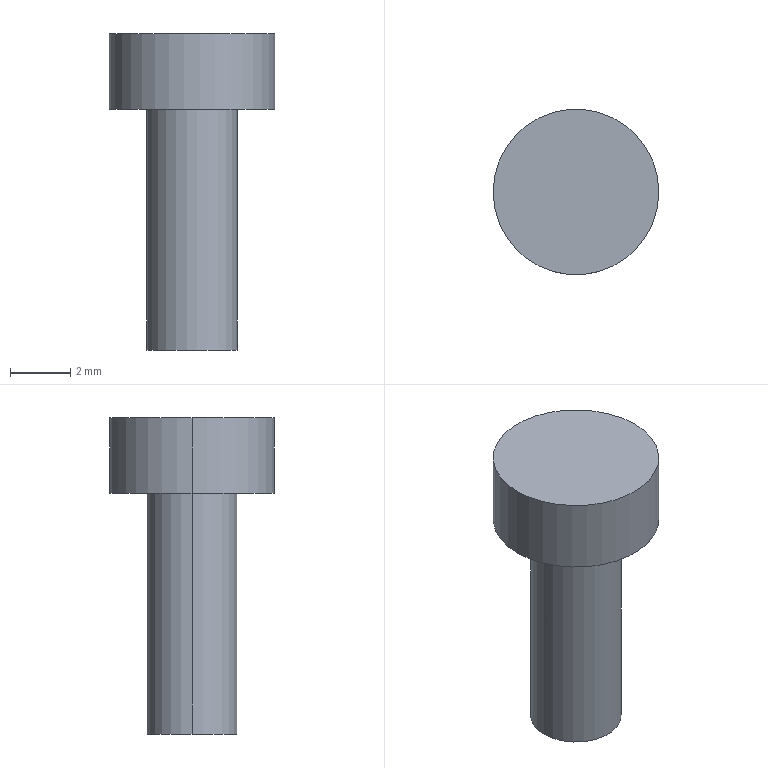Part | SolidWorks | features Extrusion 1, ICE 1 | 1 solid | 7 faces | box 5.5 x 5.5 x 10.5 mm | volume 115.944 mm3 | cylinder 4 | plane 3 | commonest cylinder face diameters 3 x2 5.5 x2
STEP:
#1=CARTESIAN_POINT('',(2.75,0.,2.5));
#2=VERTEX_POINT('',#1);
#3=CARTESIAN_POINT('',(-2.75,0.,2.5));
#4=VERTEX_POINT('',#3);
#5=CARTESIAN_POINT('',(0.,0.,2.5));
#6=DIRECTION('',(0.,0.,1.));
#7=DIRECTION('',(1.,0.,0.));
#8=AXIS2_PLACEMENT_3D('',#5,#6,#7);
#9=CIRCLE('',#8,2.75);
#10=EDGE_CURVE('',#2,#4,#9,.T.);
#11=ORIENTED_EDGE('',*,*,#10,.F.);
#12=CARTESIAN_POINT('',(2.75,0.,0.));
#13=VERTEX_POINT('',#12);
#14=CARTESIAN_POINT('',(2.75,0.,2.5));
#15=DIRECTION('',(0.,0.,-1.));
#16=VECTOR('',#15,1000.);
#17=LINE('',#14,#16);
#18=EDGE_CURVE('',#2,#13,#17,.T.);
#19=ORIENTED_EDGE('',*,*,#18,.T.);
#20=CARTESIAN_POINT('',(-2.75,0.,0.));
#21=VERTEX_POINT('',#20);
#22=CARTESIAN_POINT('',(0.,0.,0.));
#23=DIRECTION('',(0.,0.,1.));
#24=DIRECTION('',(1.,0.,0.));
#25=AXIS2_PLACEMENT_3D('',#22,#23,#24);
#26=CIRCLE('',#25,2.75);
#27=EDGE_CURVE('',#13,#21,#26,.T.);
#28=ORIENTED_EDGE('',*,*,#27,.T.);
#29=CARTESIAN_POINT('',(-2.75,0.,2.5));
#30=DIRECTION('',(0.,0.,-1.));
#31=VECTOR('',#30,1000.);
#32=LINE('',#29,#31);
#33=EDGE_CURVE('',#4,#21,#32,.T.);
#34=ORIENTED_EDGE('',*,*,#33,.F.);
#35=EDGE_LOOP('',(#11,#19,#28,#34));
#36=FACE_OUTER_BOUND('',#35,.T.);
#37=CARTESIAN_POINT('',(0.,0.,2.5));
#38=DIRECTION('',(0.,0.,-1.));
#39=DIRECTION('',(-1.,0.,0.));
#40=AXIS2_PLACEMENT_3D('',#37,#38,#39);
#41=CYLINDRICAL_SURFACE('',#40,2.75);
#42=ADVANCED_FACE('',(#36),#41,.T.);
#43=CARTESIAN_POINT('',(1.5,0.,-8.));
#44=VERTEX_POINT('',#43);
#45=CARTESIAN_POINT('',(-1.5,0.,-8.));
#46=VERTEX_POINT('',#45);
#47=CARTESIAN_POINT('',(0.,0.,-8.));
#48=DIRECTION('',(0.,0.,1.));
#49=DIRECTION('',(1.,0.,0.));
#50=AXIS2_PLACEMENT_3D('',#47,#48,#49);
#51=CIRCLE('',#50,1.5);
#52=EDGE_CURVE('',#44,#46,#51,.T.);
#53=ORIENTED_EDGE('',*,*,#52,.T.);
#54=CARTESIAN_POINT('',(-1.5,0.,0.));
#55=VERTEX_POINT('',#54);
#56=CARTESIAN_POINT('',(-1.5,0.,-8.));
#57=DIRECTION('',(0.,0.,1.));
#58=VECTOR('',#57,1000.);
#59=LINE('',#56,#58);
#60=EDGE_CURVE('',#46,#55,#59,.T.);
#61=ORIENTED_EDGE('',*,*,#60,.T.);
#62=CARTESIAN_POINT('',(1.5,0.,0.));
#63=VERTEX_POINT('',#62);
#64=CARTESIAN_POINT('',(0.,0.,0.));
#65=DIRECTION('',(0.,0.,1.));
#66=DIRECTION('',(1.,0.,0.));
#67=AXIS2_PLACEMENT_3D('',#64,#65,#66);
#68=CIRCLE('',#67,1.5);
#69=EDGE_CURVE('',#63,#55,#68,.T.);
#70=ORIENTED_EDGE('',*,*,#69,.F.);
#71=CARTESIAN_POINT('',(1.5,0.,-8.));
#72=DIRECTION('',(0.,0.,1.));
#73=VECTOR('',#72,1000.);
#74=LINE('',#71,#73);
#75=EDGE_CURVE('',#44,#63,#74,.T.);
#76=ORIENTED_EDGE('',*,*,#75,.F.);
#77=EDGE_LOOP('',(#53,#61,#70,#76));
#78=FACE_OUTER_BOUND('',#77,.T.);
#79=CARTESIAN_POINT('',(0.,0.,-8.));
#80=DIRECTION('',(0.,0.,1.));
#81=DIRECTION('',(1.,0.,0.));
#82=AXIS2_PLACEMENT_3D('',#79,#80,#81);
#83=CYLINDRICAL_SURFACE('',#82,1.5);
#84=ADVANCED_FACE('',(#78),#83,.T.);
#85=ORIENTED_EDGE('',*,*,#60,.F.);
#86=CARTESIAN_POINT('',(0.,0.,-8.));
#87=DIRECTION('',(0.,0.,1.));
#88=DIRECTION('',(1.,0.,0.));
#89=AXIS2_PLACEMENT_3D('',#86,#87,#88);
#90=CIRCLE('',#89,1.5);
#91=EDGE_CURVE('',#46,#44,#90,.T.);
#92=ORIENTED_EDGE('',*,*,#91,.T.);
#93=ORIENTED_EDGE('',*,*,#75,.T.);
#94=CARTESIAN_POINT('',(0.,0.,0.));
#95=DIRECTION('',(0.,0.,1.));
#96=DIRECTION('',(1.,0.,0.));
#97=AXIS2_PLACEMENT_3D('',#94,#95,#96);
#98=CIRCLE('',#97,1.5);
#99=EDGE_CURVE('',#55,#63,#98,.T.);
#100=ORIENTED_EDGE('',*,*,#99,.F.);
#101=EDGE_LOOP('',(#85,#92,#93,#100));
#102=FACE_OUTER_BOUND('',#101,.T.);
#103=CARTESIAN_POINT('',(0.,0.,-8.));
#104=DIRECTION('',(0.,0.,1.));
#105=DIRECTION('',(1.,0.,0.));
#106=AXIS2_PLACEMENT_3D('',#103,#104,#105);
#107=CYLINDRICAL_SURFACE('',#106,1.5);
#108=ADVANCED_FACE('',(#102),#107,.T.);
#109=ORIENTED_EDGE('',*,*,#52,.F.);
#110=ORIENTED_EDGE('',*,*,#91,.F.);
#111=EDGE_LOOP('',(#109,#110));
#112=FACE_OUTER_BOUND('',#111,.T.);
#113=CARTESIAN_POINT('',(0.,0.,-8.));
#114=DIRECTION('',(0.,0.,1.));
#115=DIRECTION('',(1.,0.,0.));
#116=AXIS2_PLACEMENT_3D('',#113,#114,#115);
#117=PLANE('',#116);
#118=ADVANCED_FACE('',(#112),#117,.F.);
#119=ORIENTED_EDGE('',*,*,#18,.F.);
#120=CARTESIAN_POINT('',(0.,0.,2.5));
#121=DIRECTION('',(0.,0.,1.));
#122=DIRECTION('',(1.,0.,0.));
#123=AXIS2_PLACEMENT_3D('',#120,#121,#122);
#124=CIRCLE('',#123,2.75);
#125=EDGE_CURVE('',#4,#2,#124,.T.);
#126=ORIENTED_EDGE('',*,*,#125,.F.);
#127=ORIENTED_EDGE('',*,*,#33,.T.);
#128=CARTESIAN_POINT('',(0.,0.,0.));
#129=DIRECTION('',(0.,0.,1.));
#130=DIRECTION('',(1.,0.,0.));
#131=AXIS2_PLACEMENT_3D('',#128,#129,#130);
#132=CIRCLE('',#131,2.75);
#133=EDGE_CURVE('',#21,#13,#132,.T.);
#134=ORIENTED_EDGE('',*,*,#133,.T.);
#135=EDGE_LOOP('',(#119,#126,#127,#134));
#136=FACE_OUTER_BOUND('',#135,.T.);
#137=CARTESIAN_POINT('',(0.,0.,2.5));
#138=DIRECTION('',(0.,0.,-1.));
#139=DIRECTION('',(-1.,0.,0.));
#140=AXIS2_PLACEMENT_3D('',#137,#138,#139);
#141=CYLINDRICAL_SURFACE('',#140,2.75);
#142=ADVANCED_FACE('',(#136),#141,.T.);
#143=ORIENTED_EDGE('',*,*,#125,.T.);
#144=ORIENTED_EDGE('',*,*,#10,.T.);
#145=EDGE_LOOP('',(#143,#144));
#146=FACE_OUTER_BOUND('',#145,.T.);
#147=CARTESIAN_POINT('',(0.,0.,2.5));
#148=DIRECTION('',(0.,0.,1.));
#149=DIRECTION('',(1.,0.,0.));
#150=AXIS2_PLACEMENT_3D('',#147,#148,#149);
#151=PLANE('',#150);
#152=ADVANCED_FACE('',(#146),#151,.T.);
#153=ORIENTED_EDGE('',*,*,#69,.T.);
#154=ORIENTED_EDGE('',*,*,#99,.T.);
#155=EDGE_LOOP('',(#153,#154));
#156=FACE_BOUND('',#155,.T.);
#157=ORIENTED_EDGE('',*,*,#133,.F.);
#158=ORIENTED_EDGE('',*,*,#27,.F.);
#159=EDGE_LOOP('',(#157,#158));
#160=FACE_OUTER_BOUND('',#159,.T.);
#161=CARTESIAN_POINT('',(0.,0.,0.));
#162=DIRECTION('',(0.,0.,1.));
#163=DIRECTION('',(1.,0.,0.));
#164=AXIS2_PLACEMENT_3D('',#161,#162,#163);
#165=PLANE('',#164);
#166=ADVANCED_FACE('',(#156,#160),#165,.F.);
#167=CLOSED_SHELL('',(#42,#84,#108,#118,#142,#152,#166));
#168=MANIFOLD_SOLID_BREP('',#167);
#169=CARTESIAN_POINT('',(0.,0.,0.));
#170=DIRECTION('',(0.,0.,1.));
#171=DIRECTION('',(1.,0.,0.));
#172=AXIS2_PLACEMENT_3D('',#169,#170,#171);
#173=(LENGTH_UNIT()NAMED_UNIT(*)SI_UNIT(.MILLI.,.METRE.));
#174=UNCERTAINTY_MEASURE_WITH_UNIT(LENGTH_MEASURE(0.00001),#173,'','');
#175=(NAMED_UNIT(*)PLANE_ANGLE_UNIT()SI_UNIT($,.RADIAN.));
#176=(NAMED_UNIT(*)SI_UNIT($,.STERADIAN.)SOLID_ANGLE_UNIT());
#177=(GEOMETRIC_REPRESENTATION_CONTEXT(3)GLOBAL_UNCERTAINTY_ASSIGNED_CONTEXT((#174))GLOBAL_UNIT_ASSIGNED_CONTEXT((#173,#175,#176))REPRESENTATION_CONTEXT('',''));
#178=ADVANCED_BREP_SHAPE_REPRESENTATION('',(#168,#172),#177);